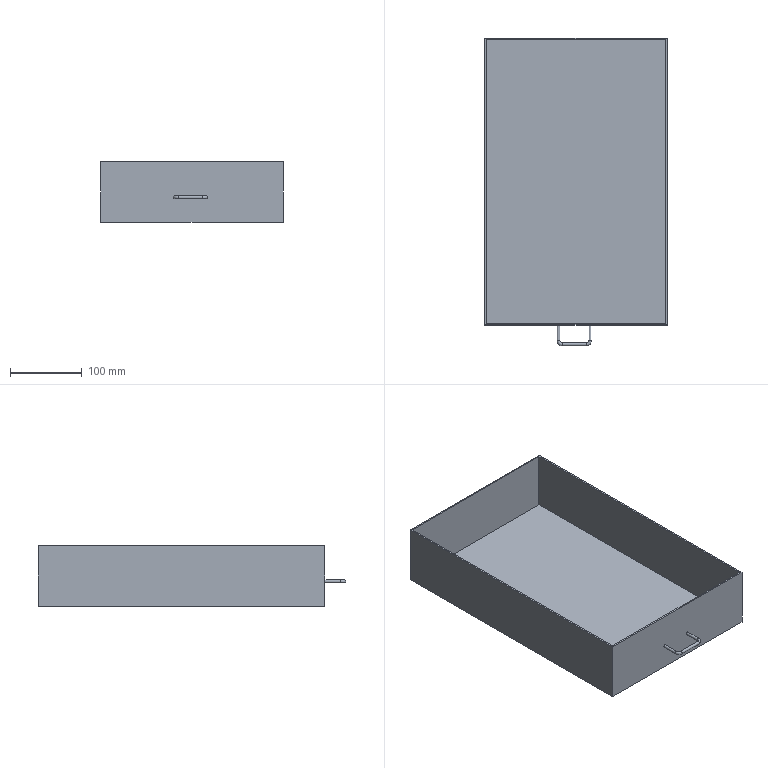Part | NX | features solid 2 | 1 solid | 16 faces | box 255 x 429 x 85 mm | volume 497676 mm3 | plane 11 | cylinder 3 | torus 2 | commonest cylinder face diameters 4 x3
STEP:
#1=CARTESIAN_POINT('',(-167.,-305.,-247.));
#2=VERTEX_POINT('',#1);
#3=CARTESIAN_POINT('',(-167.,-305.,-245.));
#4=DIRECTION('',(0.,-1.,0.));
#5=DIRECTION('',(0.,0.,-1.));
#6=AXIS2_PLACEMENT_3D('',#3,#4,#5);
#7=CIRCLE('',#6,2.);
#8=EDGE_CURVE('',#2,#2,#7,.F.);
#9=ORIENTED_EDGE('',*,*,#8,.T.);
#10=EDGE_LOOP('',(#9));
#11=FACE_BOUND('',#10,.T.);
#12=CARTESIAN_POINT('',(-270.,-305.,-195.));
#13=VERTEX_POINT('',#12);
#14=CARTESIAN_POINT('',(-15.,-305.,-195.));
#15=VERTEX_POINT('',#14);
#16=CARTESIAN_POINT('',(-235.,-305.,-195.));
#17=DIRECTION('',(1.,0.,0.));
#18=VECTOR('',#17,1000.);
#19=LINE('',#16,#18);
#20=EDGE_CURVE('',#13,#15,#19,.T.);
#21=ORIENTED_EDGE('',*,*,#20,.F.);
#22=CARTESIAN_POINT('',(-270.,-305.,-280.));
#23=VERTEX_POINT('',#22);
#24=CARTESIAN_POINT('',(-270.,-305.,-145.));
#25=DIRECTION('',(0.,0.,1.));
#26=VECTOR('',#25,1000.);
#27=LINE('',#24,#26);
#28=EDGE_CURVE('',#13,#23,#27,.F.);
#29=ORIENTED_EDGE('',*,*,#28,.T.);
#30=CARTESIAN_POINT('',(-15.,-305.,-280.));
#31=VERTEX_POINT('',#30);
#32=CARTESIAN_POINT('',(-235.,-305.,-280.));
#33=DIRECTION('',(1.,0.,0.));
#34=VECTOR('',#33,1000.);
#35=LINE('',#32,#34);
#36=EDGE_CURVE('',#23,#31,#35,.T.);
#37=ORIENTED_EDGE('',*,*,#36,.T.);
#38=CARTESIAN_POINT('',(-15.,-305.,-145.));
#39=DIRECTION('',(0.,0.,-1.));
#40=VECTOR('',#39,1000.);
#41=LINE('',#38,#40);
#42=EDGE_CURVE('',#15,#31,#41,.T.);
#43=ORIENTED_EDGE('',*,*,#42,.F.);
#44=EDGE_LOOP('',(#21,#29,#37,#43));
#45=FACE_BOUND('',#44,.T.);
#46=CARTESIAN_POINT('',(-123.,-305.,-243.));
#47=VERTEX_POINT('',#46);
#48=CARTESIAN_POINT('',(-123.,-305.,-245.));
#49=DIRECTION('',(0.,1.,0.));
#50=DIRECTION('',(0.,0.,1.));
#51=AXIS2_PLACEMENT_3D('',#48,#49,#50);
#52=CIRCLE('',#51,2.);
#53=EDGE_CURVE('',#47,#47,#52,.F.);
#54=ORIENTED_EDGE('',*,*,#53,.F.);
#55=EDGE_LOOP('',(#54));
#56=FACE_BOUND('',#55,.T.);
#57=CARTESIAN_POINT('',(-235.,-305.,-145.));
#58=DIRECTION('',(0.,1.,0.));
#59=DIRECTION('',(0.,0.,1.));
#60=AXIS2_PLACEMENT_3D('',#57,#58,#59);
#61=PLANE('',#60);
#62=ADVANCED_FACE('',(#11,#45,#56),#61,.F.);
#63=CARTESIAN_POINT('',(-15.,95.,-195.));
#64=VERTEX_POINT('',#63);
#65=CARTESIAN_POINT('',(-15.,-305.,-195.));
#66=DIRECTION('',(0.,1.,0.));
#67=VECTOR('',#66,1000.);
#68=LINE('',#65,#67);
#69=EDGE_CURVE('',#15,#64,#68,.T.);
#70=ORIENTED_EDGE('',*,*,#69,.F.);
#71=ORIENTED_EDGE('',*,*,#42,.T.);
#72=CARTESIAN_POINT('',(-15.,95.,-280.));
#73=VERTEX_POINT('',#72);
#74=CARTESIAN_POINT('',(-15.,-305.,-280.));
#75=DIRECTION('',(0.,1.,0.));
#76=VECTOR('',#75,1000.);
#77=LINE('',#74,#76);
#78=EDGE_CURVE('',#31,#73,#77,.T.);
#79=ORIENTED_EDGE('',*,*,#78,.T.);
#80=CARTESIAN_POINT('',(-15.,95.,-145.));
#81=DIRECTION('',(0.,0.,1.));
#82=VECTOR('',#81,1000.);
#83=LINE('',#80,#82);
#84=EDGE_CURVE('',#64,#73,#83,.F.);
#85=ORIENTED_EDGE('',*,*,#84,.F.);
#86=EDGE_LOOP('',(#70,#71,#79,#85));
#87=FACE_BOUND('',#86,.T.);
#88=CARTESIAN_POINT('',(-15.,-305.,-145.));
#89=DIRECTION('',(-1.,0.,0.));
#90=DIRECTION('',(0.,0.,1.));
#91=AXIS2_PLACEMENT_3D('',#88,#89,#90);
#92=PLANE('',#91);
#93=ADVANCED_FACE('',(#87),#92,.F.);
#94=CARTESIAN_POINT('',(-270.,95.,-195.));
#95=VERTEX_POINT('',#94);
#96=CARTESIAN_POINT('',(-270.,405.,-195.));
#97=DIRECTION('',(0.,1.,0.));
#98=VECTOR('',#97,1000.);
#99=LINE('',#96,#98);
#100=EDGE_CURVE('',#95,#13,#99,.F.);
#101=ORIENTED_EDGE('',*,*,#100,.F.);
#102=CARTESIAN_POINT('',(-270.,95.,-280.));
#103=VERTEX_POINT('',#102);
#104=CARTESIAN_POINT('',(-270.,95.,-125.));
#105=DIRECTION('',(0.,0.,-1.));
#106=VECTOR('',#105,1000.);
#107=LINE('',#104,#106);
#108=EDGE_CURVE('',#95,#103,#107,.T.);
#109=ORIENTED_EDGE('',*,*,#108,.T.);
#110=CARTESIAN_POINT('',(-270.,405.,-280.));
#111=DIRECTION('',(0.,1.,0.));
#112=VECTOR('',#111,1000.);
#113=LINE('',#110,#112);
#114=EDGE_CURVE('',#103,#23,#113,.F.);
#115=ORIENTED_EDGE('',*,*,#114,.T.);
#116=ORIENTED_EDGE('',*,*,#28,.F.);
#117=EDGE_LOOP('',(#101,#109,#115,#116));
#118=FACE_BOUND('',#117,.T.);
#119=CARTESIAN_POINT('',(-270.,405.,-375.));
#120=DIRECTION('',(-1.,0.,0.));
#121=DIRECTION('',(0.,0.,1.));
#122=AXIS2_PLACEMENT_3D('',#119,#120,#121);
#123=PLANE('',#122);
#124=ADVANCED_FACE('',(#118),#123,.T.);
#125=CARTESIAN_POINT('',(0.,95.,-195.));
#126=DIRECTION('',(1.,0.,0.));
#127=VECTOR('',#126,1000.);
#128=LINE('',#125,#127);
#129=EDGE_CURVE('',#64,#95,#128,.F.);
#130=ORIENTED_EDGE('',*,*,#129,.F.);
#131=ORIENTED_EDGE('',*,*,#84,.T.);
#132=CARTESIAN_POINT('',(-17.5,95.,-280.));
#133=DIRECTION('',(1.,0.,0.));
#134=VECTOR('',#133,1000.);
#135=LINE('',#132,#134);
#136=EDGE_CURVE('',#73,#103,#135,.F.);
#137=ORIENTED_EDGE('',*,*,#136,.T.);
#138=ORIENTED_EDGE('',*,*,#108,.F.);
#139=EDGE_LOOP('',(#130,#131,#137,#138));
#140=FACE_BOUND('',#139,.T.);
#141=CARTESIAN_POINT('',(-640.,95.,-125.));
#142=DIRECTION('',(0.,-1.,0.));
#143=DIRECTION('',(1.,0.,0.));
#144=AXIS2_PLACEMENT_3D('',#141,#142,#143);
#145=PLANE('',#144);
#146=ADVANCED_FACE('',(#140),#145,.F.);
#147=ORIENTED_EDGE('',*,*,#136,.F.);
#148=ORIENTED_EDGE('',*,*,#78,.F.);
#149=ORIENTED_EDGE('',*,*,#36,.F.);
#150=ORIENTED_EDGE('',*,*,#114,.F.);
#151=EDGE_LOOP('',(#147,#148,#149,#150));
#152=FACE_BOUND('',#151,.T.);
#153=CARTESIAN_POINT('',(-17.5,47.5,-280.));
#154=DIRECTION('',(0.,0.,1.));
#155=DIRECTION('',(1.,0.,0.));
#156=AXIS2_PLACEMENT_3D('',#153,#154,#155);
#157=PLANE('',#156);
#158=ADVANCED_FACE('',(#152),#157,.F.);
#159=CARTESIAN_POINT('',(-17.5,-302.5,-195.));
#160=VERTEX_POINT('',#159);
#161=CARTESIAN_POINT('',(-268.,-302.5,-195.));
#162=VERTEX_POINT('',#161);
#163=CARTESIAN_POINT('',(-15.,-302.5,-195.));
#164=DIRECTION('',(-1.,0.,0.));
#165=VECTOR('',#164,1000.);
#166=LINE('',#163,#165);
#167=EDGE_CURVE('',#160,#162,#166,.T.);
#168=ORIENTED_EDGE('',*,*,#167,.T.);
#169=CARTESIAN_POINT('',(-268.,93.,-195.));
#170=VERTEX_POINT('',#169);
#171=CARTESIAN_POINT('',(-268.,-302.5,-195.));
#172=DIRECTION('',(0.,1.,0.));
#173=VECTOR('',#172,1000.);
#174=LINE('',#171,#173);
#175=EDGE_CURVE('',#162,#170,#174,.T.);
#176=ORIENTED_EDGE('',*,*,#175,.T.);
#177=CARTESIAN_POINT('',(-17.5,93.,-195.));
#178=VERTEX_POINT('',#177);
#179=CARTESIAN_POINT('',(-235.,93.,-195.));
#180=DIRECTION('',(1.,0.,0.));
#181=VECTOR('',#180,1000.);
#182=LINE('',#179,#181);
#183=EDGE_CURVE('',#170,#178,#182,.T.);
#184=ORIENTED_EDGE('',*,*,#183,.T.);
#185=CARTESIAN_POINT('',(-17.5,47.5,-195.));
#186=DIRECTION('',(0.,-1.,0.));
#187=VECTOR('',#186,1000.);
#188=LINE('',#185,#187);
#189=EDGE_CURVE('',#178,#160,#188,.T.);
#190=ORIENTED_EDGE('',*,*,#189,.T.);
#191=EDGE_LOOP('',(#168,#176,#184,#190));
#192=FACE_BOUND('',#191,.T.);
#193=ORIENTED_EDGE('',*,*,#100,.T.);
#194=ORIENTED_EDGE('',*,*,#20,.T.);
#195=ORIENTED_EDGE('',*,*,#69,.T.);
#196=ORIENTED_EDGE('',*,*,#129,.T.);
#197=EDGE_LOOP('',(#193,#194,#195,#196));
#198=FACE_BOUND('',#197,.T.);
#199=CARTESIAN_POINT('',(0.,0.,-195.));
#200=DIRECTION('',(0.,0.,1.));
#201=DIRECTION('',(1.,0.,0.));
#202=AXIS2_PLACEMENT_3D('',#199,#200,#201);
#203=PLANE('',#202);
#204=ADVANCED_FACE('',(#192,#198),#203,.T.);
#205=CARTESIAN_POINT('',(-17.5,-302.5,-277.5));
#206=VERTEX_POINT('',#205);
#207=CARTESIAN_POINT('',(-17.5,93.,-277.5));
#208=VERTEX_POINT('',#207);
#209=CARTESIAN_POINT('',(-17.5,-302.5,-277.5));
#210=DIRECTION('',(0.,1.,0.));
#211=VECTOR('',#210,1000.);
#212=LINE('',#209,#211);
#213=EDGE_CURVE('',#206,#208,#212,.T.);
#214=ORIENTED_EDGE('',*,*,#213,.T.);
#215=CARTESIAN_POINT('',(-268.,93.,-277.5));
#216=VERTEX_POINT('',#215);
#217=CARTESIAN_POINT('',(-17.5,93.,-277.5));
#218=DIRECTION('',(-1.,0.,0.));
#219=VECTOR('',#218,1000.);
#220=LINE('',#217,#219);
#221=EDGE_CURVE('',#208,#216,#220,.T.);
#222=ORIENTED_EDGE('',*,*,#221,.T.);
#223=CARTESIAN_POINT('',(-268.,-302.5,-277.5));
#224=VERTEX_POINT('',#223);
#225=CARTESIAN_POINT('',(-268.,47.5,-277.5));
#226=DIRECTION('',(0.,-1.,0.));
#227=VECTOR('',#226,1000.);
#228=LINE('',#225,#227);
#229=EDGE_CURVE('',#216,#224,#228,.T.);
#230=ORIENTED_EDGE('',*,*,#229,.T.);
#231=CARTESIAN_POINT('',(-232.5,-302.5,-277.5));
#232=DIRECTION('',(1.,0.,0.));
#233=VECTOR('',#232,1000.);
#234=LINE('',#231,#233);
#235=EDGE_CURVE('',#224,#206,#234,.T.);
#236=ORIENTED_EDGE('',*,*,#235,.T.);
#237=EDGE_LOOP('',(#214,#222,#230,#236));
#238=FACE_BOUND('',#237,.T.);
#239=CARTESIAN_POINT('',(-17.5,47.5,-277.5));
#240=DIRECTION('',(0.,0.,1.));
#241=DIRECTION('',(1.,0.,0.));
#242=AXIS2_PLACEMENT_3D('',#239,#240,#241);
#243=PLANE('',#242);
#244=ADVANCED_FACE('',(#238),#243,.T.);
#245=ORIENTED_EDGE('',*,*,#189,.F.);
#246=CARTESIAN_POINT('',(-17.5,93.,-145.));
#247=DIRECTION('',(0.,0.,-1.));
#248=VECTOR('',#247,1000.);
#249=LINE('',#246,#248);
#250=EDGE_CURVE('',#178,#208,#249,.T.);
#251=ORIENTED_EDGE('',*,*,#250,.T.);
#252=ORIENTED_EDGE('',*,*,#213,.F.);
#253=CARTESIAN_POINT('',(-17.5,-302.5,-145.));
#254=DIRECTION('',(0.,0.,-1.));
#255=VECTOR('',#254,1000.);
#256=LINE('',#253,#255);
#257=EDGE_CURVE('',#160,#206,#256,.T.);
#258=ORIENTED_EDGE('',*,*,#257,.F.);
#259=EDGE_LOOP('',(#245,#251,#252,#258));
#260=FACE_BOUND('',#259,.T.);
#261=CARTESIAN_POINT('',(-17.5,47.5,-145.));
#262=DIRECTION('',(1.,0.,0.));
#263=DIRECTION('',(0.,0.,-1.));
#264=AXIS2_PLACEMENT_3D('',#261,#262,#263);
#265=PLANE('',#264);
#266=ADVANCED_FACE('',(#260),#265,.F.);
#267=ORIENTED_EDGE('',*,*,#175,.F.);
#268=CARTESIAN_POINT('',(-268.,-302.5,-145.));
#269=DIRECTION('',(0.,0.,-1.));
#270=VECTOR('',#269,1000.);
#271=LINE('',#268,#270);
#272=EDGE_CURVE('',#162,#224,#271,.T.);
#273=ORIENTED_EDGE('',*,*,#272,.T.);
#274=ORIENTED_EDGE('',*,*,#229,.F.);
#275=CARTESIAN_POINT('',(-268.,93.,-145.));
#276=DIRECTION('',(0.,0.,-1.));
#277=VECTOR('',#276,1000.);
#278=LINE('',#275,#277);
#279=EDGE_CURVE('',#170,#216,#278,.T.);
#280=ORIENTED_EDGE('',*,*,#279,.F.);
#281=EDGE_LOOP('',(#267,#273,#274,#280));
#282=FACE_BOUND('',#281,.T.);
#283=CARTESIAN_POINT('',(-268.,-302.5,-145.));
#284=DIRECTION('',(-1.,0.,0.));
#285=DIRECTION('',(0.,0.,1.));
#286=AXIS2_PLACEMENT_3D('',#283,#284,#285);
#287=PLANE('',#286);
#288=ADVANCED_FACE('',(#282),#287,.F.);
#289=ORIENTED_EDGE('',*,*,#183,.F.);
#290=ORIENTED_EDGE('',*,*,#279,.T.);
#291=ORIENTED_EDGE('',*,*,#221,.F.);
#292=ORIENTED_EDGE('',*,*,#250,.F.);
#293=EDGE_LOOP('',(#289,#290,#291,#292));
#294=FACE_BOUND('',#293,.T.);
#295=CARTESIAN_POINT('',(-235.,93.,-145.));
#296=DIRECTION('',(0.,1.,0.));
#297=DIRECTION('',(0.,0.,1.));
#298=AXIS2_PLACEMENT_3D('',#295,#296,#297);
#299=PLANE('',#298);
#300=ADVANCED_FACE('',(#294),#299,.F.);
#301=ORIENTED_EDGE('',*,*,#167,.F.);
#302=ORIENTED_EDGE('',*,*,#257,.T.);
#303=ORIENTED_EDGE('',*,*,#235,.F.);
#304=ORIENTED_EDGE('',*,*,#272,.F.);
#305=EDGE_LOOP('',(#301,#302,#303,#304));
#306=FACE_BOUND('',#305,.T.);
#307=CARTESIAN_POINT('',(-15.,-302.5,-145.));
#308=DIRECTION('',(0.,-1.,0.));
#309=DIRECTION('',(0.,0.,-1.));
#310=AXIS2_PLACEMENT_3D('',#307,#308,#309);
#311=PLANE('',#310);
#312=ADVANCED_FACE('',(#306),#311,.F.);
#313=CARTESIAN_POINT('',(-162.,-332.,-247.));
#314=VERTEX_POINT('',#313);
#315=CARTESIAN_POINT('',(-162.,-332.,-245.));
#316=DIRECTION('',(-1.,0.,0.));
#317=DIRECTION('',(0.,0.,-1.));
#318=AXIS2_PLACEMENT_3D('',#315,#316,#317);
#319=CIRCLE('',#318,2.);
#320=EDGE_CURVE('',#314,#314,#319,.T.);
#321=ORIENTED_EDGE('',*,*,#320,.T.);
#322=EDGE_LOOP('',(#321));
#323=FACE_BOUND('',#322,.T.);
#324=CARTESIAN_POINT('',(-167.,-327.,-247.));
#325=VERTEX_POINT('',#324);
#326=CARTESIAN_POINT('',(-167.,-327.,-245.));
#327=DIRECTION('',(0.,1.,0.));
#328=DIRECTION('',(0.,0.,-1.));
#329=AXIS2_PLACEMENT_3D('',#326,#327,#328);
#330=CIRCLE('',#329,2.);
#331=EDGE_CURVE('',#325,#325,#330,.T.);
#332=ORIENTED_EDGE('',*,*,#331,.F.);
#333=EDGE_LOOP('',(#332));
#334=FACE_BOUND('',#333,.T.);
#335=CARTESIAN_POINT('',(-162.,-327.,-245.));
#336=DIRECTION('',(0.,0.,-1.));
#337=DIRECTION('',(-1.,0.,0.));
#338=AXIS2_PLACEMENT_3D('',#335,#336,#337);
#339=TOROIDAL_SURFACE('',#338,5.,2.);
#340=ADVANCED_FACE('',(#323,#334),#339,.T.);
#341=ORIENTED_EDGE('',*,*,#331,.T.);
#342=EDGE_LOOP('',(#341));
#343=FACE_BOUND('',#342,.T.);
#344=ORIENTED_EDGE('',*,*,#8,.F.);
#345=EDGE_LOOP('',(#344));
#346=FACE_BOUND('',#345,.T.);
#347=CARTESIAN_POINT('',(-167.,-327.,-245.));
#348=DIRECTION('',(0.,1.,0.));
#349=DIRECTION('',(0.,0.,1.));
#350=AXIS2_PLACEMENT_3D('',#347,#348,#349);
#351=CYLINDRICAL_SURFACE('',#350,2.);
#352=ADVANCED_FACE('',(#343,#346),#351,.T.);
#353=CARTESIAN_POINT('',(-128.,-332.,-247.));
#354=VERTEX_POINT('',#353);
#355=CARTESIAN_POINT('',(-128.,-332.,-245.));
#356=DIRECTION('',(-1.,0.,0.));
#357=DIRECTION('',(0.,0.,-1.));
#358=AXIS2_PLACEMENT_3D('',#355,#356,#357);
#359=CIRCLE('',#358,2.);
#360=EDGE_CURVE('',#354,#354,#359,.T.);
#361=ORIENTED_EDGE('',*,*,#360,.T.);
#362=EDGE_LOOP('',(#361));
#363=FACE_BOUND('',#362,.T.);
#364=ORIENTED_EDGE('',*,*,#320,.F.);
#365=EDGE_LOOP('',(#364));
#366=FACE_BOUND('',#365,.T.);
#367=CARTESIAN_POINT('',(-128.,-332.,-245.));
#368=DIRECTION('',(-1.,0.,0.));
#369=DIRECTION('',(0.,0.,1.));
#370=AXIS2_PLACEMENT_3D('',#367,#368,#369);
#371=CYLINDRICAL_SURFACE('',#370,2.);
#372=ADVANCED_FACE('',(#363,#366),#371,.T.);
#373=CARTESIAN_POINT('',(-123.,-327.,-247.));
#374=VERTEX_POINT('',#373);
#375=CARTESIAN_POINT('',(-123.,-327.,-245.));
#376=DIRECTION('',(0.,-1.,0.));
#377=DIRECTION('',(0.,0.,-1.));
#378=AXIS2_PLACEMENT_3D('',#375,#376,#377);
#379=CIRCLE('',#378,2.);
#380=EDGE_CURVE('',#374,#374,#379,.T.);
#381=ORIENTED_EDGE('',*,*,#380,.T.);
#382=EDGE_LOOP('',(#381));
#383=FACE_BOUND('',#382,.T.);
#384=ORIENTED_EDGE('',*,*,#360,.F.);
#385=EDGE_LOOP('',(#384));
#386=FACE_BOUND('',#385,.T.);
#387=CARTESIAN_POINT('',(-128.,-327.,-245.));
#388=DIRECTION('',(0.,0.,-1.));
#389=DIRECTION('',(-1.,0.,0.));
#390=AXIS2_PLACEMENT_3D('',#387,#388,#389);
#391=TOROIDAL_SURFACE('',#390,5.,2.);
#392=ADVANCED_FACE('',(#383,#386),#391,.T.);
#393=ORIENTED_EDGE('',*,*,#380,.F.);
#394=EDGE_LOOP('',(#393));
#395=FACE_BOUND('',#394,.T.);
#396=ORIENTED_EDGE('',*,*,#53,.T.);
#397=EDGE_LOOP('',(#396));
#398=FACE_BOUND('',#397,.T.);
#399=CARTESIAN_POINT('',(-123.,-327.,-245.));
#400=DIRECTION('',(0.,1.,0.));
#401=DIRECTION('',(0.,0.,1.));
#402=AXIS2_PLACEMENT_3D('',#399,#400,#401);
#403=CYLINDRICAL_SURFACE('',#402,2.);
#404=ADVANCED_FACE('',(#395,#398),#403,.T.);
#405=CLOSED_SHELL('',(#62,#93,#124,#146,#158,#204,#244,#266,#288,#300,#312,#340,#352,#372,#392,#404));
#406=MANIFOLD_SOLID_BREP('',#405);
#407=(LENGTH_UNIT()NAMED_UNIT(*)SI_UNIT(.MILLI.,.METRE.));
#408=UNCERTAINTY_MEASURE_WITH_UNIT(LENGTH_MEASURE(0.00001),#407,'','');
#409=(NAMED_UNIT(*)PLANE_ANGLE_UNIT()SI_UNIT($,.RADIAN.));
#410=(NAMED_UNIT(*)SI_UNIT($,.STERADIAN.)SOLID_ANGLE_UNIT());
#411=(GEOMETRIC_REPRESENTATION_CONTEXT(3)GLOBAL_UNCERTAINTY_ASSIGNED_CONTEXT((#408))GLOBAL_UNIT_ASSIGNED_CONTEXT((#407,#409,#410))REPRESENTATION_CONTEXT('',''));
#412=ADVANCED_BREP_SHAPE_REPRESENTATION('',(#406),#411);